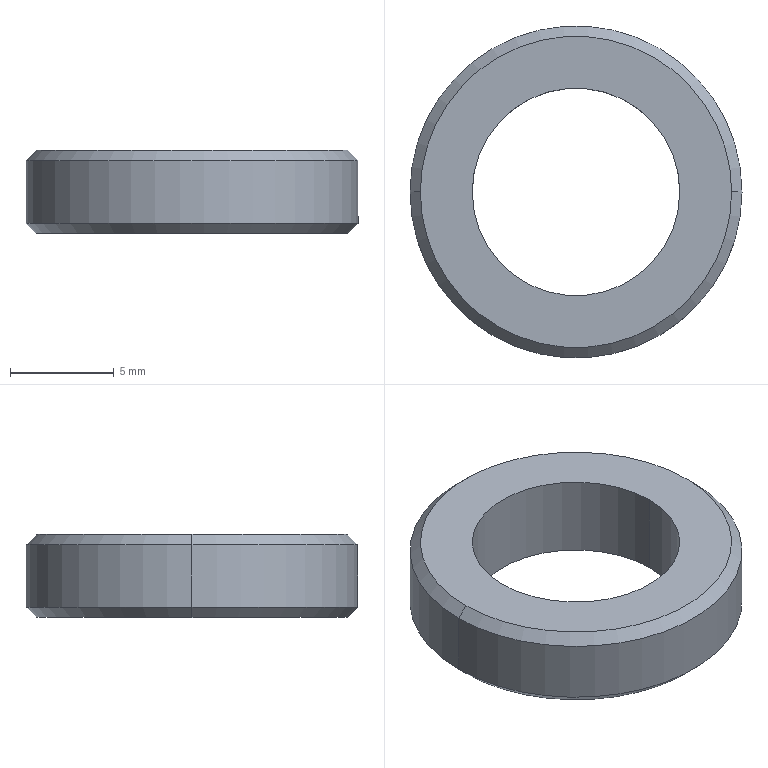Part | SolidWorks | features Revolution 1 | 1 solid | 10 faces | box 16 x 16 x 4 mm | volume 477.784 mm3 | cone 4 | cylinder 4 | plane 2 | commonest cylinder face diameters 10 x2 16 x2
STEP:
#1=CARTESIAN_POINT('',(-7.5,0.,4.));
#2=VERTEX_POINT('',#1);
#3=CARTESIAN_POINT('',(7.5,0.,4.));
#4=VERTEX_POINT('',#3);
#5=CARTESIAN_POINT('',(0.,0.,4.));
#6=DIRECTION('',(0.,0.,-1.));
#7=DIRECTION('',(-1.,0.,0.));
#8=AXIS2_PLACEMENT_3D('',#5,#6,#7);
#9=CIRCLE('',#8,7.5);
#10=EDGE_CURVE('',#2,#4,#9,.T.);
#11=ORIENTED_EDGE('',*,*,#10,.T.);
#12=CARTESIAN_POINT('',(8.,0.,3.5));
#13=VERTEX_POINT('',#12);
#14=CARTESIAN_POINT('',(8.,0.,3.5));
#15=DIRECTION('',(0.7071,0.,-0.7071));
#16=VECTOR('',#15,1000.);
#17=LINE('',#14,#16);
#18=EDGE_CURVE('',#4,#13,#17,.T.);
#19=ORIENTED_EDGE('',*,*,#18,.T.);
#20=CARTESIAN_POINT('',(-8.,0.,3.5));
#21=VERTEX_POINT('',#20);
#22=CARTESIAN_POINT('',(0.,0.,3.5));
#23=DIRECTION('',(0.,0.,-1.));
#24=DIRECTION('',(-1.,0.,0.));
#25=AXIS2_PLACEMENT_3D('',#22,#23,#24);
#26=CIRCLE('',#25,8.);
#27=EDGE_CURVE('',#21,#13,#26,.T.);
#28=ORIENTED_EDGE('',*,*,#27,.F.);
#29=CARTESIAN_POINT('',(-8.,0.,3.5));
#30=DIRECTION('',(-0.7071,0.,-0.7071));
#31=VECTOR('',#30,1000.);
#32=LINE('',#29,#31);
#33=EDGE_CURVE('',#2,#21,#32,.T.);
#34=ORIENTED_EDGE('',*,*,#33,.F.);
#35=EDGE_LOOP('',(#11,#19,#28,#34));
#36=FACE_OUTER_BOUND('',#35,.T.);
#37=CARTESIAN_POINT('',(0.,0.,3.5));
#38=DIRECTION('',(0.,0.,-1.));
#39=DIRECTION('',(-1.,0.,0.));
#40=AXIS2_PLACEMENT_3D('',#37,#38,#39);
#41=CONICAL_SURFACE('',#40,8.,0.7854);
#42=ADVANCED_FACE('',(#36),#41,.T.);
#43=ORIENTED_EDGE('',*,*,#27,.T.);
#44=CARTESIAN_POINT('',(8.,0.,0.5));
#45=VERTEX_POINT('',#44);
#46=CARTESIAN_POINT('',(8.,0.,4.));
#47=DIRECTION('',(0.,0.,-1.));
#48=VECTOR('',#47,1000.);
#49=LINE('',#46,#48);
#50=EDGE_CURVE('',#13,#45,#49,.T.);
#51=ORIENTED_EDGE('',*,*,#50,.T.);
#52=CARTESIAN_POINT('',(-8.,0.,0.5));
#53=VERTEX_POINT('',#52);
#54=CARTESIAN_POINT('',(0.,0.,0.5));
#55=DIRECTION('',(0.,0.,-1.));
#56=DIRECTION('',(-1.,0.,0.));
#57=AXIS2_PLACEMENT_3D('',#54,#55,#56);
#58=CIRCLE('',#57,8.);
#59=EDGE_CURVE('',#53,#45,#58,.T.);
#60=ORIENTED_EDGE('',*,*,#59,.F.);
#61=CARTESIAN_POINT('',(-8.,0.,4.));
#62=DIRECTION('',(0.,0.,-1.));
#63=VECTOR('',#62,1000.);
#64=LINE('',#61,#63);
#65=EDGE_CURVE('',#21,#53,#64,.T.);
#66=ORIENTED_EDGE('',*,*,#65,.F.);
#67=EDGE_LOOP('',(#43,#51,#60,#66));
#68=FACE_OUTER_BOUND('',#67,.T.);
#69=CARTESIAN_POINT('',(0.,0.,4.));
#70=DIRECTION('',(0.,0.,-1.));
#71=DIRECTION('',(-1.,0.,0.));
#72=AXIS2_PLACEMENT_3D('',#69,#70,#71);
#73=CYLINDRICAL_SURFACE('',#72,8.);
#74=ADVANCED_FACE('',(#68),#73,.T.);
#75=CARTESIAN_POINT('',(-7.5,0.,0.));
#76=VERTEX_POINT('',#75);
#77=CARTESIAN_POINT('',(7.5,0.,0.));
#78=VERTEX_POINT('',#77);
#79=CARTESIAN_POINT('',(0.,0.,0.));
#80=DIRECTION('',(0.,0.,-1.));
#81=DIRECTION('',(-1.,0.,0.));
#82=AXIS2_PLACEMENT_3D('',#79,#80,#81);
#83=CIRCLE('',#82,7.5);
#84=EDGE_CURVE('',#76,#78,#83,.T.);
#85=ORIENTED_EDGE('',*,*,#84,.F.);
#86=CARTESIAN_POINT('',(-7.5,0.,0.));
#87=DIRECTION('',(-0.7071,0.,0.7071));
#88=VECTOR('',#87,1000.);
#89=LINE('',#86,#88);
#90=EDGE_CURVE('',#76,#53,#89,.T.);
#91=ORIENTED_EDGE('',*,*,#90,.T.);
#92=ORIENTED_EDGE('',*,*,#59,.T.);
#93=CARTESIAN_POINT('',(7.5,0.,0.));
#94=DIRECTION('',(0.7071,0.,0.7071));
#95=VECTOR('',#94,1000.);
#96=LINE('',#93,#95);
#97=EDGE_CURVE('',#78,#45,#96,.T.);
#98=ORIENTED_EDGE('',*,*,#97,.F.);
#99=EDGE_LOOP('',(#85,#91,#92,#98));
#100=FACE_OUTER_BOUND('',#99,.T.);
#101=CARTESIAN_POINT('',(0.,0.,0.));
#102=DIRECTION('',(0.,0.,1.));
#103=DIRECTION('',(1.,0.,0.));
#104=AXIS2_PLACEMENT_3D('',#101,#102,#103);
#105=CONICAL_SURFACE('',#104,7.5,0.7854);
#106=ADVANCED_FACE('',(#100),#105,.T.);
#107=CARTESIAN_POINT('',(5.,0.,4.));
#108=VERTEX_POINT('',#107);
#109=CARTESIAN_POINT('',(-5.,0.,4.));
#110=VERTEX_POINT('',#109);
#111=CARTESIAN_POINT('',(0.,0.,4.));
#112=DIRECTION('',(0.,0.,-1.));
#113=DIRECTION('',(-1.,0.,0.));
#114=AXIS2_PLACEMENT_3D('',#111,#112,#113);
#115=CIRCLE('',#114,5.);
#116=EDGE_CURVE('',#108,#110,#115,.T.);
#117=ORIENTED_EDGE('',*,*,#116,.F.);
#118=CARTESIAN_POINT('',(5.,0.,0.));
#119=VERTEX_POINT('',#118);
#120=CARTESIAN_POINT('',(5.,0.,4.));
#121=DIRECTION('',(0.,0.,-1.));
#122=VECTOR('',#121,1000.);
#123=LINE('',#120,#122);
#124=EDGE_CURVE('',#108,#119,#123,.T.);
#125=ORIENTED_EDGE('',*,*,#124,.T.);
#126=CARTESIAN_POINT('',(-5.,0.,0.));
#127=VERTEX_POINT('',#126);
#128=CARTESIAN_POINT('',(0.,0.,0.));
#129=DIRECTION('',(0.,0.,-1.));
#130=DIRECTION('',(-1.,0.,0.));
#131=AXIS2_PLACEMENT_3D('',#128,#129,#130);
#132=CIRCLE('',#131,5.);
#133=EDGE_CURVE('',#119,#127,#132,.T.);
#134=ORIENTED_EDGE('',*,*,#133,.T.);
#135=CARTESIAN_POINT('',(-5.,0.,4.));
#136=DIRECTION('',(0.,0.,-1.));
#137=VECTOR('',#136,1000.);
#138=LINE('',#135,#137);
#139=EDGE_CURVE('',#110,#127,#138,.T.);
#140=ORIENTED_EDGE('',*,*,#139,.F.);
#141=EDGE_LOOP('',(#117,#125,#134,#140));
#142=FACE_OUTER_BOUND('',#141,.T.);
#143=CARTESIAN_POINT('',(0.,0.,4.));
#144=DIRECTION('',(0.,0.,-1.));
#145=DIRECTION('',(-1.,0.,0.));
#146=AXIS2_PLACEMENT_3D('',#143,#144,#145);
#147=CYLINDRICAL_SURFACE('',#146,5.);
#148=ADVANCED_FACE('',(#142),#147,.F.);
#149=CARTESIAN_POINT('',(0.,0.,4.));
#150=DIRECTION('',(0.,0.,-1.));
#151=DIRECTION('',(-1.,0.,0.));
#152=AXIS2_PLACEMENT_3D('',#149,#150,#151);
#153=CIRCLE('',#152,5.);
#154=EDGE_CURVE('',#110,#108,#153,.T.);
#155=ORIENTED_EDGE('',*,*,#154,.T.);
#156=ORIENTED_EDGE('',*,*,#116,.T.);
#157=EDGE_LOOP('',(#155,#156));
#158=FACE_BOUND('',#157,.T.);
#159=ORIENTED_EDGE('',*,*,#10,.F.);
#160=CARTESIAN_POINT('',(0.,0.,4.));
#161=DIRECTION('',(0.,0.,-1.));
#162=DIRECTION('',(-1.,0.,0.));
#163=AXIS2_PLACEMENT_3D('',#160,#161,#162);
#164=CIRCLE('',#163,7.5);
#165=EDGE_CURVE('',#4,#2,#164,.T.);
#166=ORIENTED_EDGE('',*,*,#165,.F.);
#167=EDGE_LOOP('',(#159,#166));
#168=FACE_OUTER_BOUND('',#167,.T.);
#169=CARTESIAN_POINT('',(7.5,0.,4.));
#170=DIRECTION('',(0.,0.,1.));
#171=DIRECTION('',(1.,0.,0.));
#172=AXIS2_PLACEMENT_3D('',#169,#170,#171);
#173=PLANE('',#172);
#174=ADVANCED_FACE('',(#158,#168),#173,.T.);
#175=ORIENTED_EDGE('',*,*,#124,.F.);
#176=ORIENTED_EDGE('',*,*,#154,.F.);
#177=ORIENTED_EDGE('',*,*,#139,.T.);
#178=CARTESIAN_POINT('',(0.,0.,0.));
#179=DIRECTION('',(0.,0.,-1.));
#180=DIRECTION('',(-1.,0.,0.));
#181=AXIS2_PLACEMENT_3D('',#178,#179,#180);
#182=CIRCLE('',#181,5.);
#183=EDGE_CURVE('',#127,#119,#182,.T.);
#184=ORIENTED_EDGE('',*,*,#183,.T.);
#185=EDGE_LOOP('',(#175,#176,#177,#184));
#186=FACE_OUTER_BOUND('',#185,.T.);
#187=CARTESIAN_POINT('',(0.,0.,4.));
#188=DIRECTION('',(0.,0.,-1.));
#189=DIRECTION('',(-1.,0.,0.));
#190=AXIS2_PLACEMENT_3D('',#187,#188,#189);
#191=CYLINDRICAL_SURFACE('',#190,5.);
#192=ADVANCED_FACE('',(#186),#191,.F.);
#193=CARTESIAN_POINT('',(0.,0.,0.));
#194=DIRECTION('',(0.,0.,-1.));
#195=DIRECTION('',(-1.,0.,0.));
#196=AXIS2_PLACEMENT_3D('',#193,#194,#195);
#197=CIRCLE('',#196,7.5);
#198=EDGE_CURVE('',#78,#76,#197,.T.);
#199=ORIENTED_EDGE('',*,*,#198,.T.);
#200=ORIENTED_EDGE('',*,*,#84,.T.);
#201=EDGE_LOOP('',(#199,#200));
#202=FACE_OUTER_BOUND('',#201,.T.);
#203=ORIENTED_EDGE('',*,*,#183,.F.);
#204=ORIENTED_EDGE('',*,*,#133,.F.);
#205=EDGE_LOOP('',(#203,#204));
#206=FACE_BOUND('',#205,.T.);
#207=CARTESIAN_POINT('',(5.,0.,0.));
#208=DIRECTION('',(0.,0.,-1.));
#209=DIRECTION('',(-1.,0.,0.));
#210=AXIS2_PLACEMENT_3D('',#207,#208,#209);
#211=PLANE('',#210);
#212=ADVANCED_FACE('',(#202,#206),#211,.T.);
#213=ORIENTED_EDGE('',*,*,#90,.F.);
#214=ORIENTED_EDGE('',*,*,#198,.F.);
#215=ORIENTED_EDGE('',*,*,#97,.T.);
#216=CARTESIAN_POINT('',(0.,0.,0.5));
#217=DIRECTION('',(0.,0.,-1.));
#218=DIRECTION('',(-1.,0.,0.));
#219=AXIS2_PLACEMENT_3D('',#216,#217,#218);
#220=CIRCLE('',#219,8.);
#221=EDGE_CURVE('',#45,#53,#220,.T.);
#222=ORIENTED_EDGE('',*,*,#221,.T.);
#223=EDGE_LOOP('',(#213,#214,#215,#222));
#224=FACE_OUTER_BOUND('',#223,.T.);
#225=CARTESIAN_POINT('',(0.,0.,0.));
#226=DIRECTION('',(0.,0.,1.));
#227=DIRECTION('',(1.,0.,0.));
#228=AXIS2_PLACEMENT_3D('',#225,#226,#227);
#229=CONICAL_SURFACE('',#228,7.5,0.7854);
#230=ADVANCED_FACE('',(#224),#229,.T.);
#231=ORIENTED_EDGE('',*,*,#50,.F.);
#232=CARTESIAN_POINT('',(0.,0.,3.5));
#233=DIRECTION('',(0.,0.,-1.));
#234=DIRECTION('',(-1.,0.,0.));
#235=AXIS2_PLACEMENT_3D('',#232,#233,#234);
#236=CIRCLE('',#235,8.);
#237=EDGE_CURVE('',#13,#21,#236,.T.);
#238=ORIENTED_EDGE('',*,*,#237,.T.);
#239=ORIENTED_EDGE('',*,*,#65,.T.);
#240=ORIENTED_EDGE('',*,*,#221,.F.);
#241=EDGE_LOOP('',(#231,#238,#239,#240));
#242=FACE_OUTER_BOUND('',#241,.T.);
#243=CARTESIAN_POINT('',(0.,0.,4.));
#244=DIRECTION('',(0.,0.,-1.));
#245=DIRECTION('',(-1.,0.,0.));
#246=AXIS2_PLACEMENT_3D('',#243,#244,#245);
#247=CYLINDRICAL_SURFACE('',#246,8.);
#248=ADVANCED_FACE('',(#242),#247,.T.);
#249=ORIENTED_EDGE('',*,*,#18,.F.);
#250=ORIENTED_EDGE('',*,*,#165,.T.);
#251=ORIENTED_EDGE('',*,*,#33,.T.);
#252=ORIENTED_EDGE('',*,*,#237,.F.);
#253=EDGE_LOOP('',(#249,#250,#251,#252));
#254=FACE_OUTER_BOUND('',#253,.T.);
#255=CARTESIAN_POINT('',(0.,0.,3.5));
#256=DIRECTION('',(0.,0.,-1.));
#257=DIRECTION('',(-1.,0.,0.));
#258=AXIS2_PLACEMENT_3D('',#255,#256,#257);
#259=CONICAL_SURFACE('',#258,8.,0.7854);
#260=ADVANCED_FACE('',(#254),#259,.T.);
#261=CLOSED_SHELL('',(#42,#74,#106,#148,#174,#192,#212,#230,#248,#260));
#262=MANIFOLD_SOLID_BREP('',#261);
#263=CARTESIAN_POINT('',(0.,0.,0.));
#264=DIRECTION('',(0.,0.,1.));
#265=DIRECTION('',(1.,0.,0.));
#266=AXIS2_PLACEMENT_3D('',#263,#264,#265);
#267=(LENGTH_UNIT()NAMED_UNIT(*)SI_UNIT(.MILLI.,.METRE.));
#268=UNCERTAINTY_MEASURE_WITH_UNIT(LENGTH_MEASURE(0.00001),#267,'','');
#269=(NAMED_UNIT(*)PLANE_ANGLE_UNIT()SI_UNIT($,.RADIAN.));
#270=(NAMED_UNIT(*)SI_UNIT($,.STERADIAN.)SOLID_ANGLE_UNIT());
#271=(GEOMETRIC_REPRESENTATION_CONTEXT(3)GLOBAL_UNCERTAINTY_ASSIGNED_CONTEXT((#268))GLOBAL_UNIT_ASSIGNED_CONTEXT((#267,#269,#270))REPRESENTATION_CONTEXT('',''));
#272=ADVANCED_BREP_SHAPE_REPRESENTATION('',(#262,#266),#271);